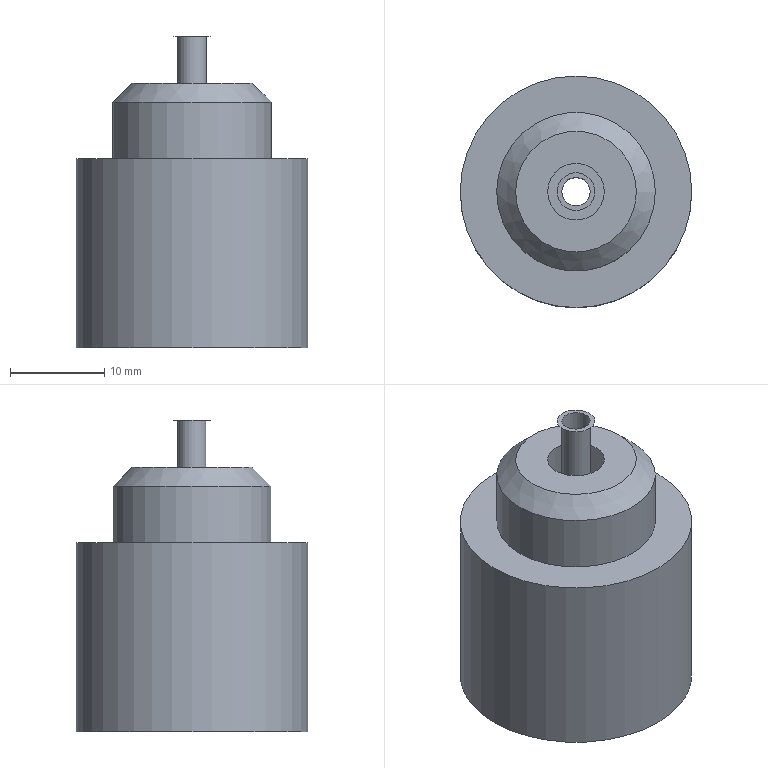Part | NX | features BREP 1, DATUM_CSYS 1 | 1 solid | 11 faces | box 24.5 x 24.5 x 33 mm | volume 10618 mm3 | plane 5 | cylinder 4 | cone 2 | commonest cylinder face diameters 3 x1 6.24 x1 16.8 x1 24.5 x1
STEP:
#1=CARTESIAN_POINT('',(12.25,0.,0.));
#2=VERTEX_POINT('',#1);
#3=CARTESIAN_POINT('',(0.,0.,0.));
#4=DIRECTION('',(0.,0.,1.));
#5=DIRECTION('',(1.,0.,0.));
#6=AXIS2_PLACEMENT_3D('',#3,#4,#5);
#7=CIRCLE('',#6,12.25);
#8=EDGE_CURVE('',#2,#2,#7,.T.);
#9=ORIENTED_EDGE('',*,*,#8,.F.);
#10=EDGE_LOOP('',(#9));
#11=FACE_BOUND('',#10,.T.);
#12=CARTESIAN_POINT('',(3.12,0.,0.));
#13=VERTEX_POINT('',#12);
#14=CARTESIAN_POINT('',(0.,0.,0.));
#15=DIRECTION('',(0.,0.,1.));
#16=DIRECTION('',(1.,0.,0.));
#17=AXIS2_PLACEMENT_3D('',#14,#15,#16);
#18=CIRCLE('',#17,3.12);
#19=EDGE_CURVE('',#13,#13,#18,.T.);
#20=ORIENTED_EDGE('',*,*,#19,.T.);
#21=EDGE_LOOP('',(#20));
#22=FACE_BOUND('',#21,.T.);
#23=CARTESIAN_POINT('',(0.,0.,0.));
#24=DIRECTION('',(0.,0.,1.));
#25=DIRECTION('',(-1.,0.,0.));
#26=AXIS2_PLACEMENT_3D('',#23,#24,#25);
#27=PLANE('',#26);
#28=ADVANCED_FACE('',(#11,#22),#27,.F.);
#29=CARTESIAN_POINT('',(12.25,0.,20.));
#30=VERTEX_POINT('',#29);
#31=CARTESIAN_POINT('',(0.,0.,20.));
#32=DIRECTION('',(0.,0.,1.));
#33=DIRECTION('',(1.,0.,0.));
#34=AXIS2_PLACEMENT_3D('',#31,#32,#33);
#35=CIRCLE('',#34,12.25);
#36=EDGE_CURVE('',#30,#30,#35,.T.);
#37=ORIENTED_EDGE('',*,*,#36,.T.);
#38=EDGE_LOOP('',(#37));
#39=FACE_BOUND('',#38,.T.);
#40=CARTESIAN_POINT('',(8.4,0.,20.));
#41=VERTEX_POINT('',#40);
#42=CARTESIAN_POINT('',(0.,0.,20.));
#43=DIRECTION('',(0.,0.,1.));
#44=DIRECTION('',(1.,0.,0.));
#45=AXIS2_PLACEMENT_3D('',#42,#43,#44);
#46=CIRCLE('',#45,8.4);
#47=EDGE_CURVE('',#41,#41,#46,.T.);
#48=ORIENTED_EDGE('',*,*,#47,.F.);
#49=EDGE_LOOP('',(#48));
#50=FACE_BOUND('',#49,.T.);
#51=CARTESIAN_POINT('',(0.,0.,20.));
#52=DIRECTION('',(0.,0.,1.));
#53=DIRECTION('',(-1.,0.,0.));
#54=AXIS2_PLACEMENT_3D('',#51,#52,#53);
#55=PLANE('',#54);
#56=ADVANCED_FACE('',(#39,#50),#55,.T.);
#57=ORIENTED_EDGE('',*,*,#8,.T.);
#58=CARTESIAN_POINT('',(12.25,0.,0.));
#59=DIRECTION('',(0.,0.,1.));
#60=VECTOR('',#59,1000.);
#61=LINE('',#58,#60);
#62=EDGE_CURVE('',#2,#30,#61,.T.);
#63=ORIENTED_EDGE('',*,*,#62,.T.);
#64=ORIENTED_EDGE('',*,*,#36,.F.);
#65=ORIENTED_EDGE('',*,*,#62,.F.);
#66=EDGE_LOOP('',(#57,#63,#64,#65));
#67=FACE_BOUND('',#66,.T.);
#68=CARTESIAN_POINT('',(0.,0.,0.));
#69=DIRECTION('',(0.,0.,1.));
#70=DIRECTION('',(-1.,0.,0.));
#71=AXIS2_PLACEMENT_3D('',#68,#69,#70);
#72=CYLINDRICAL_SURFACE('',#71,12.25);
#73=ADVANCED_FACE('',(#67),#72,.T.);
#74=ORIENTED_EDGE('',*,*,#47,.T.);
#75=CARTESIAN_POINT('',(8.4,0.,26.));
#76=VERTEX_POINT('',#75);
#77=CARTESIAN_POINT('',(8.4,0.,20.));
#78=DIRECTION('',(0.,0.,1.));
#79=VECTOR('',#78,1000.);
#80=LINE('',#77,#79);
#81=EDGE_CURVE('',#41,#76,#80,.T.);
#82=ORIENTED_EDGE('',*,*,#81,.T.);
#83=CARTESIAN_POINT('',(0.,0.,26.));
#84=DIRECTION('',(0.,0.,-1.));
#85=DIRECTION('',(1.,0.,0.));
#86=AXIS2_PLACEMENT_3D('',#83,#84,#85);
#87=CIRCLE('',#86,8.4);
#88=EDGE_CURVE('',#76,#76,#87,.T.);
#89=ORIENTED_EDGE('',*,*,#88,.T.);
#90=ORIENTED_EDGE('',*,*,#81,.F.);
#91=EDGE_LOOP('',(#74,#82,#89,#90));
#92=FACE_BOUND('',#91,.T.);
#93=CARTESIAN_POINT('',(0.,0.,20.));
#94=DIRECTION('',(0.,0.,1.));
#95=DIRECTION('',(-1.,0.,0.));
#96=AXIS2_PLACEMENT_3D('',#93,#94,#95);
#97=CYLINDRICAL_SURFACE('',#96,8.4);
#98=ADVANCED_FACE('',(#92),#97,.T.);
#99=CARTESIAN_POINT('',(6.4,0.,28.));
#100=VERTEX_POINT('',#99);
#101=CARTESIAN_POINT('',(0.,0.,28.));
#102=DIRECTION('',(0.,0.,-1.));
#103=DIRECTION('',(1.,0.,0.));
#104=AXIS2_PLACEMENT_3D('',#101,#102,#103);
#105=CIRCLE('',#104,6.4);
#106=EDGE_CURVE('',#100,#100,#105,.T.);
#107=ORIENTED_EDGE('',*,*,#106,.F.);
#108=EDGE_LOOP('',(#107));
#109=FACE_BOUND('',#108,.T.);
#110=CARTESIAN_POINT('',(3.,0.,28.));
#111=VERTEX_POINT('',#110);
#112=CARTESIAN_POINT('',(0.,0.,28.));
#113=DIRECTION('',(0.,0.,1.));
#114=DIRECTION('',(1.,0.,0.));
#115=AXIS2_PLACEMENT_3D('',#112,#113,#114);
#116=CIRCLE('',#115,3.);
#117=EDGE_CURVE('',#111,#111,#116,.T.);
#118=ORIENTED_EDGE('',*,*,#117,.F.);
#119=EDGE_LOOP('',(#118));
#120=FACE_BOUND('',#119,.T.);
#121=CARTESIAN_POINT('',(0.,0.,28.));
#122=DIRECTION('',(0.,0.,1.));
#123=DIRECTION('',(-1.,0.,0.));
#124=AXIS2_PLACEMENT_3D('',#121,#122,#123);
#125=PLANE('',#124);
#126=ADVANCED_FACE('',(#109,#120),#125,.T.);
#127=ORIENTED_EDGE('',*,*,#117,.T.);
#128=CARTESIAN_POINT('',(2.,0.,33.));
#129=VERTEX_POINT('',#128);
#130=CARTESIAN_POINT('',(3.,0.,28.));
#131=DIRECTION('',(-0.1961,0.,0.9806));
#132=VECTOR('',#131,1000.);
#133=LINE('',#130,#132);
#134=EDGE_CURVE('',#111,#129,#133,.T.);
#135=ORIENTED_EDGE('',*,*,#134,.T.);
#136=CARTESIAN_POINT('',(0.,0.,33.));
#137=DIRECTION('',(0.,0.,1.));
#138=DIRECTION('',(1.,0.,0.));
#139=AXIS2_PLACEMENT_3D('',#136,#137,#138);
#140=CIRCLE('',#139,2.);
#141=EDGE_CURVE('',#129,#129,#140,.T.);
#142=ORIENTED_EDGE('',*,*,#141,.F.);
#143=ORIENTED_EDGE('',*,*,#134,.F.);
#144=EDGE_LOOP('',(#127,#135,#142,#143));
#145=FACE_BOUND('',#144,.T.);
#146=CARTESIAN_POINT('',(0.,0.,33.));
#147=DIRECTION('',(0.,0.,-1.));
#148=DIRECTION('',(-1.,0.,0.));
#149=AXIS2_PLACEMENT_3D('',#146,#147,#148);
#150=CONICAL_SURFACE('',#149,2.,0.1974);
#151=ADVANCED_FACE('',(#145),#150,.T.);
#152=ORIENTED_EDGE('',*,*,#141,.T.);
#153=EDGE_LOOP('',(#152));
#154=FACE_BOUND('',#153,.T.);
#155=CARTESIAN_POINT('',(1.5,0.,33.));
#156=VERTEX_POINT('',#155);
#157=CARTESIAN_POINT('',(0.,0.,33.));
#158=DIRECTION('',(0.,0.,-1.));
#159=DIRECTION('',(1.,0.,0.));
#160=AXIS2_PLACEMENT_3D('',#157,#158,#159);
#161=CIRCLE('',#160,1.5);
#162=EDGE_CURVE('',#156,#156,#161,.T.);
#163=ORIENTED_EDGE('',*,*,#162,.T.);
#164=EDGE_LOOP('',(#163));
#165=FACE_BOUND('',#164,.T.);
#166=CARTESIAN_POINT('',(0.,0.,33.));
#167=DIRECTION('',(0.,0.,1.));
#168=DIRECTION('',(-1.,0.,0.));
#169=AXIS2_PLACEMENT_3D('',#166,#167,#168);
#170=PLANE('',#169);
#171=ADVANCED_FACE('',(#154,#165),#170,.T.);
#172=CARTESIAN_POINT('',(1.5,0.,15.));
#173=VERTEX_POINT('',#172);
#174=CARTESIAN_POINT('',(1.5,0.,33.));
#175=DIRECTION('',(0.,0.,-1.));
#176=VECTOR('',#175,1000.);
#177=LINE('',#174,#176);
#178=EDGE_CURVE('',#156,#173,#177,.T.);
#179=ORIENTED_EDGE('',*,*,#178,.T.);
#180=CARTESIAN_POINT('',(0.,0.,15.));
#181=DIRECTION('',(0.,0.,1.));
#182=DIRECTION('',(1.,0.,0.));
#183=AXIS2_PLACEMENT_3D('',#180,#181,#182);
#184=CIRCLE('',#183,1.5);
#185=EDGE_CURVE('',#173,#173,#184,.T.);
#186=ORIENTED_EDGE('',*,*,#185,.F.);
#187=ORIENTED_EDGE('',*,*,#178,.F.);
#188=ORIENTED_EDGE('',*,*,#162,.F.);
#189=EDGE_LOOP('',(#179,#186,#187,#188));
#190=FACE_BOUND('',#189,.T.);
#191=CARTESIAN_POINT('',(0.,0.,33.));
#192=DIRECTION('',(0.,0.,-1.));
#193=DIRECTION('',(-1.,0.,0.));
#194=AXIS2_PLACEMENT_3D('',#191,#192,#193);
#195=CYLINDRICAL_SURFACE('',#194,1.5);
#196=ADVANCED_FACE('',(#190),#195,.F.);
#197=CARTESIAN_POINT('',(6.4,0.,28.));
#198=DIRECTION('',(0.7071,0.,-0.7071));
#199=VECTOR('',#198,1000.);
#200=LINE('',#197,#199);
#201=EDGE_CURVE('',#100,#76,#200,.T.);
#202=ORIENTED_EDGE('',*,*,#201,.T.);
#203=ORIENTED_EDGE('',*,*,#88,.F.);
#204=ORIENTED_EDGE('',*,*,#201,.F.);
#205=ORIENTED_EDGE('',*,*,#106,.T.);
#206=EDGE_LOOP('',(#202,#203,#204,#205));
#207=FACE_BOUND('',#206,.T.);
#208=CARTESIAN_POINT('',(0.,0.,28.));
#209=DIRECTION('',(0.,0.,-1.));
#210=DIRECTION('',(-1.,0.,0.));
#211=AXIS2_PLACEMENT_3D('',#208,#209,#210);
#212=CONICAL_SURFACE('',#211,6.4,0.7854);
#213=ADVANCED_FACE('',(#207),#212,.T.);
#214=CARTESIAN_POINT('',(3.12,0.,15.));
#215=VERTEX_POINT('',#214);
#216=CARTESIAN_POINT('',(3.12,0.,0.));
#217=DIRECTION('',(0.,0.,1.));
#218=VECTOR('',#217,1000.);
#219=LINE('',#216,#218);
#220=EDGE_CURVE('',#13,#215,#219,.T.);
#221=ORIENTED_EDGE('',*,*,#220,.T.);
#222=CARTESIAN_POINT('',(0.,0.,15.));
#223=DIRECTION('',(0.,0.,1.));
#224=DIRECTION('',(1.,0.,0.));
#225=AXIS2_PLACEMENT_3D('',#222,#223,#224);
#226=CIRCLE('',#225,3.12);
#227=EDGE_CURVE('',#215,#215,#226,.T.);
#228=ORIENTED_EDGE('',*,*,#227,.T.);
#229=ORIENTED_EDGE('',*,*,#220,.F.);
#230=ORIENTED_EDGE('',*,*,#19,.F.);
#231=EDGE_LOOP('',(#221,#228,#229,#230));
#232=FACE_BOUND('',#231,.T.);
#233=CARTESIAN_POINT('',(0.,0.,0.));
#234=DIRECTION('',(0.,0.,1.));
#235=DIRECTION('',(-1.,0.,0.));
#236=AXIS2_PLACEMENT_3D('',#233,#234,#235);
#237=CYLINDRICAL_SURFACE('',#236,3.12);
#238=ADVANCED_FACE('',(#232),#237,.F.);
#239=ORIENTED_EDGE('',*,*,#227,.F.);
#240=EDGE_LOOP('',(#239));
#241=FACE_BOUND('',#240,.T.);
#242=ORIENTED_EDGE('',*,*,#185,.T.);
#243=EDGE_LOOP('',(#242));
#244=FACE_BOUND('',#243,.T.);
#245=CARTESIAN_POINT('',(0.,0.,15.));
#246=DIRECTION('',(0.,0.,1.));
#247=DIRECTION('',(-1.,0.,0.));
#248=AXIS2_PLACEMENT_3D('',#245,#246,#247);
#249=PLANE('',#248);
#250=ADVANCED_FACE('',(#241,#244),#249,.F.);
#251=CLOSED_SHELL('',(#28,#56,#73,#98,#126,#151,#171,#196,#213,#238,#250));
#252=MANIFOLD_SOLID_BREP('',#251);
#253=(LENGTH_UNIT()NAMED_UNIT(*)SI_UNIT(.MILLI.,.METRE.));
#254=UNCERTAINTY_MEASURE_WITH_UNIT(LENGTH_MEASURE(0.00001),#253,'','');
#255=(NAMED_UNIT(*)PLANE_ANGLE_UNIT()SI_UNIT($,.RADIAN.));
#256=(NAMED_UNIT(*)SI_UNIT($,.STERADIAN.)SOLID_ANGLE_UNIT());
#257=(GEOMETRIC_REPRESENTATION_CONTEXT(3)GLOBAL_UNCERTAINTY_ASSIGNED_CONTEXT((#254))GLOBAL_UNIT_ASSIGNED_CONTEXT((#253,#255,#256))REPRESENTATION_CONTEXT('',''));
#258=ADVANCED_BREP_SHAPE_REPRESENTATION('',(#252),#257);